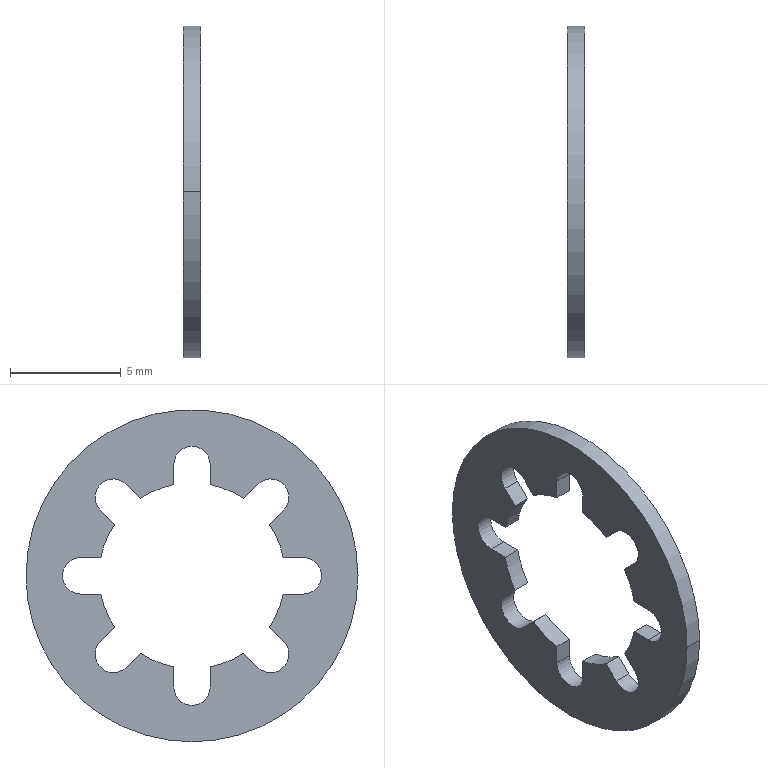Part | 1 solid | 36 faces | box 0.8 x 15 x 15 mm | volume 81.196 mm3 | cylinder 18 | plane 18 | commonest cylinder face diameters 1.65 x8 8.4 x8 15 x2
STEP:
#1=CARTESIAN_POINT('',(0.,0.,0.));
#2=DIRECTION('',(0.,0.,1.));
#3=DIRECTION('',(1.,0.,0.));
#4=AXIS2_PLACEMENT_3D('',#1,#2,#3);
#5=CARTESIAN_POINT('',(-282.773,180.5,-203.374));
#6=VERTEX_POINT('',#5);
#7=CARTESIAN_POINT('',(-283.573,180.5,-203.374));
#8=VERTEX_POINT('',#7);
#9=CARTESIAN_POINT('',(-282.773,180.5,-203.374));
#10=DIRECTION('',(-1.,0.,0.));
#11=VECTOR('',#10,1.);
#12=LINE('',#9,#11);
#13=EDGE_CURVE('',#6,#8,#12,.T.);
#14=ORIENTED_EDGE('',*,*,#13,.F.);
#15=CARTESIAN_POINT('',(-282.773,173.,-210.874));
#16=VERTEX_POINT('',#15);
#17=CARTESIAN_POINT('',(-282.773,173.,-203.374));
#18=DIRECTION('',(-1.,0.,0.));
#19=DIRECTION('',(0.,0.,-1.));
#20=AXIS2_PLACEMENT_3D('',#17,#18,#19);
#21=CIRCLE('',#20,7.5);
#22=EDGE_CURVE('',#6,#16,#21,.T.);
#23=ORIENTED_EDGE('',*,*,#22,.T.);
#24=CARTESIAN_POINT('',(-282.773,165.5,-203.374));
#25=VERTEX_POINT('',#24);
#26=CARTESIAN_POINT('',(-282.773,173.,-203.374));
#27=DIRECTION('',(-1.,0.,0.));
#28=DIRECTION('',(0.,0.,-1.));
#29=AXIS2_PLACEMENT_3D('',#26,#27,#28);
#30=CIRCLE('',#29,7.5);
#31=EDGE_CURVE('',#16,#25,#30,.T.);
#32=ORIENTED_EDGE('',*,*,#31,.T.);
#33=CARTESIAN_POINT('',(-283.573,165.5,-203.374));
#34=VERTEX_POINT('',#33);
#35=CARTESIAN_POINT('',(-282.773,165.5,-203.374));
#36=DIRECTION('',(-1.,0.,0.));
#37=VECTOR('',#36,1.);
#38=LINE('',#35,#37);
#39=EDGE_CURVE('',#25,#34,#38,.T.);
#40=ORIENTED_EDGE('',*,*,#39,.T.);
#41=CARTESIAN_POINT('',(-283.573,173.,-210.874));
#42=VERTEX_POINT('',#41);
#43=CARTESIAN_POINT('',(-283.573,173.,-203.374));
#44=DIRECTION('',(-1.,0.,0.));
#45=DIRECTION('',(0.,0.,-1.));
#46=AXIS2_PLACEMENT_3D('',#43,#44,#45);
#47=CIRCLE('',#46,7.5);
#48=EDGE_CURVE('',#42,#34,#47,.T.);
#49=ORIENTED_EDGE('',*,*,#48,.F.);
#50=CARTESIAN_POINT('',(-283.573,173.,-203.374));
#51=DIRECTION('',(-1.,0.,0.));
#52=DIRECTION('',(0.,0.,-1.));
#53=AXIS2_PLACEMENT_3D('',#50,#51,#52);
#54=CIRCLE('',#53,7.5);
#55=EDGE_CURVE('',#8,#42,#54,.T.);
#56=ORIENTED_EDGE('',*,*,#55,.F.);
#57=EDGE_LOOP('',(#14,#23,#32,#40,#49,#56));
#58=FACE_OUTER_BOUND('',#57,.T.);
#59=CARTESIAN_POINT('',(-283.573,173.,-203.374));
#60=DIRECTION('',(-1.,0.,0.));
#61=DIRECTION('',(0.,0.,1.));
#62=AXIS2_PLACEMENT_3D('',#59,#60,#61);
#63=CYLINDRICAL_SURFACE('',#62,7.5);
#64=ADVANCED_FACE('',(#58),#63,.T.);
#65=ORIENTED_EDGE('',*,*,#22,.F.);
#66=CARTESIAN_POINT('',(-282.773,173.,-203.374));
#67=DIRECTION('',(-1.,0.,0.));
#68=DIRECTION('',(0.,0.,-1.));
#69=AXIS2_PLACEMENT_3D('',#66,#67,#68);
#70=CIRCLE('',#69,7.5);
#71=EDGE_CURVE('',#25,#6,#70,.T.);
#72=ORIENTED_EDGE('',*,*,#71,.F.);
#73=ORIENTED_EDGE('',*,*,#31,.F.);
#74=EDGE_LOOP('',(#65,#72,#73));
#75=FACE_OUTER_BOUND('',#74,.T.);
#76=CARTESIAN_POINT('',(-282.773,172.175,-199.256));
#77=VERTEX_POINT('',#76);
#78=CARTESIAN_POINT('',(-282.773,170.671,-199.879));
#79=VERTEX_POINT('',#78);
#80=CARTESIAN_POINT('',(-282.773,173.,-203.374));
#81=DIRECTION('',(1.,0.,0.));
#82=DIRECTION('',(0.,-0.5544,0.8322));
#83=AXIS2_PLACEMENT_3D('',#80,#81,#82);
#84=CIRCLE('',#83,4.2);
#85=EDGE_CURVE('',#77,#79,#84,.T.);
#86=ORIENTED_EDGE('',*,*,#85,.F.);
#87=CARTESIAN_POINT('',(-282.773,172.175,-198.349));
#88=VERTEX_POINT('',#87);
#89=CARTESIAN_POINT('',(-282.773,172.175,-199.256));
#90=DIRECTION('',(0.,0.,-1.));
#91=VECTOR('',#90,1.);
#92=LINE('',#89,#91);
#93=EDGE_CURVE('',#88,#77,#92,.T.);
#94=ORIENTED_EDGE('',*,*,#93,.F.);
#95=CARTESIAN_POINT('',(-282.773,173.825,-198.349));
#96=VERTEX_POINT('',#95);
#97=CARTESIAN_POINT('',(-282.773,173.,-198.349));
#98=DIRECTION('',(1.,0.,0.));
#99=DIRECTION('',(0.,-1.,0.));
#100=AXIS2_PLACEMENT_3D('',#97,#98,#99);
#101=CIRCLE('',#100,0.825);
#102=EDGE_CURVE('',#96,#88,#101,.T.);
#103=ORIENTED_EDGE('',*,*,#102,.F.);
#104=CARTESIAN_POINT('',(-282.773,173.825,-199.256));
#105=VERTEX_POINT('',#104);
#106=CARTESIAN_POINT('',(-282.773,173.825,-198.349));
#107=DIRECTION('',(0.,0.,1.));
#108=VECTOR('',#107,1.);
#109=LINE('',#106,#108);
#110=EDGE_CURVE('',#105,#96,#109,.T.);
#111=ORIENTED_EDGE('',*,*,#110,.F.);
#112=CARTESIAN_POINT('',(-282.773,175.329,-199.879));
#113=VERTEX_POINT('',#112);
#114=CARTESIAN_POINT('',(-282.773,173.,-203.374));
#115=DIRECTION('',(1.,0.,0.));
#116=DIRECTION('',(0.,0.1964,0.9805));
#117=AXIS2_PLACEMENT_3D('',#114,#115,#116);
#118=CIRCLE('',#117,4.2);
#119=EDGE_CURVE('',#113,#105,#118,.T.);
#120=ORIENTED_EDGE('',*,*,#119,.F.);
#121=CARTESIAN_POINT('',(-282.773,175.97,-199.238));
#122=VERTEX_POINT('',#121);
#123=CARTESIAN_POINT('',(-282.773,175.329,-199.879));
#124=DIRECTION('',(0.,-0.7071,-0.7071));
#125=VECTOR('',#124,1.);
#126=LINE('',#123,#125);
#127=EDGE_CURVE('',#122,#113,#126,.T.);
#128=ORIENTED_EDGE('',*,*,#127,.F.);
#129=CARTESIAN_POINT('',(-282.773,177.137,-200.404));
#130=VERTEX_POINT('',#129);
#131=CARTESIAN_POINT('',(-282.773,176.553,-199.821));
#132=DIRECTION('',(1.,0.,0.));
#133=DIRECTION('',(0.,-0.7071,0.7071));
#134=AXIS2_PLACEMENT_3D('',#131,#132,#133);
#135=CIRCLE('',#134,0.825);
#136=EDGE_CURVE('',#130,#122,#135,.T.);
#137=ORIENTED_EDGE('',*,*,#136,.F.);
#138=CARTESIAN_POINT('',(-282.773,176.495,-201.046));
#139=VERTEX_POINT('',#138);
#140=CARTESIAN_POINT('',(-282.773,177.137,-200.404));
#141=DIRECTION('',(0.,0.7071,0.7071));
#142=VECTOR('',#141,1.);
#143=LINE('',#140,#142);
#144=EDGE_CURVE('',#139,#130,#143,.T.);
#145=ORIENTED_EDGE('',*,*,#144,.F.);
#146=CARTESIAN_POINT('',(-282.773,177.118,-202.549));
#147=VERTEX_POINT('',#146);
#148=CARTESIAN_POINT('',(-282.773,173.,-203.374));
#149=DIRECTION('',(1.,0.,0.));
#150=DIRECTION('',(0.,0.8322,0.5544));
#151=AXIS2_PLACEMENT_3D('',#148,#149,#150);
#152=CIRCLE('',#151,4.2);
#153=EDGE_CURVE('',#147,#139,#152,.T.);
#154=ORIENTED_EDGE('',*,*,#153,.F.);
#155=CARTESIAN_POINT('',(-282.773,178.025,-202.549));
#156=VERTEX_POINT('',#155);
#157=CARTESIAN_POINT('',(-282.773,177.118,-202.549));
#158=DIRECTION('',(0.,-1.,0.));
#159=VECTOR('',#158,1.);
#160=LINE('',#157,#159);
#161=EDGE_CURVE('',#156,#147,#160,.T.);
#162=ORIENTED_EDGE('',*,*,#161,.F.);
#163=CARTESIAN_POINT('',(-282.773,178.025,-204.199));
#164=VERTEX_POINT('',#163);
#165=CARTESIAN_POINT('',(-282.773,178.025,-203.374));
#166=DIRECTION('',(1.,0.,0.));
#167=DIRECTION('',(0.,0.,1.));
#168=AXIS2_PLACEMENT_3D('',#165,#166,#167);
#169=CIRCLE('',#168,0.825);
#170=EDGE_CURVE('',#164,#156,#169,.T.);
#171=ORIENTED_EDGE('',*,*,#170,.F.);
#172=CARTESIAN_POINT('',(-282.773,177.118,-204.199));
#173=VERTEX_POINT('',#172);
#174=CARTESIAN_POINT('',(-282.773,178.025,-204.199));
#175=DIRECTION('',(0.,1.,0.));
#176=VECTOR('',#175,1.);
#177=LINE('',#174,#176);
#178=EDGE_CURVE('',#173,#164,#177,.T.);
#179=ORIENTED_EDGE('',*,*,#178,.F.);
#180=CARTESIAN_POINT('',(-282.773,176.495,-205.703));
#181=VERTEX_POINT('',#180);
#182=CARTESIAN_POINT('',(-282.773,173.,-203.374));
#183=DIRECTION('',(1.,0.,0.));
#184=DIRECTION('',(0.,0.9805,-0.1964));
#185=AXIS2_PLACEMENT_3D('',#182,#183,#184);
#186=CIRCLE('',#185,4.2);
#187=EDGE_CURVE('',#181,#173,#186,.T.);
#188=ORIENTED_EDGE('',*,*,#187,.F.);
#189=CARTESIAN_POINT('',(-282.773,177.137,-206.344));
#190=VERTEX_POINT('',#189);
#191=CARTESIAN_POINT('',(-282.773,176.495,-205.703));
#192=DIRECTION('',(0.,-0.7071,0.7071));
#193=VECTOR('',#192,1.);
#194=LINE('',#191,#193);
#195=EDGE_CURVE('',#190,#181,#194,.T.);
#196=ORIENTED_EDGE('',*,*,#195,.F.);
#197=CARTESIAN_POINT('',(-282.773,175.97,-207.511));
#198=VERTEX_POINT('',#197);
#199=CARTESIAN_POINT('',(-282.773,176.553,-206.927));
#200=DIRECTION('',(1.,0.,0.));
#201=DIRECTION('',(0.,0.7071,0.7071));
#202=AXIS2_PLACEMENT_3D('',#199,#200,#201);
#203=CIRCLE('',#202,0.825);
#204=EDGE_CURVE('',#198,#190,#203,.T.);
#205=ORIENTED_EDGE('',*,*,#204,.F.);
#206=CARTESIAN_POINT('',(-282.773,175.329,-206.87));
#207=VERTEX_POINT('',#206);
#208=CARTESIAN_POINT('',(-282.773,175.97,-207.511));
#209=DIRECTION('',(0.,0.7071,-0.7071));
#210=VECTOR('',#209,1.);
#211=LINE('',#208,#210);
#212=EDGE_CURVE('',#207,#198,#211,.T.);
#213=ORIENTED_EDGE('',*,*,#212,.F.);
#214=CARTESIAN_POINT('',(-282.773,173.825,-207.492));
#215=VERTEX_POINT('',#214);
#216=CARTESIAN_POINT('',(-282.773,173.,-203.374));
#217=DIRECTION('',(1.,0.,0.));
#218=DIRECTION('',(0.,0.5544,-0.8322));
#219=AXIS2_PLACEMENT_3D('',#216,#217,#218);
#220=CIRCLE('',#219,4.2);
#221=EDGE_CURVE('',#215,#207,#220,.T.);
#222=ORIENTED_EDGE('',*,*,#221,.F.);
#223=CARTESIAN_POINT('',(-282.773,173.825,-208.399));
#224=VERTEX_POINT('',#223);
#225=CARTESIAN_POINT('',(-282.773,173.825,-207.492));
#226=DIRECTION('',(0.,0.,1.));
#227=VECTOR('',#226,1.);
#228=LINE('',#225,#227);
#229=EDGE_CURVE('',#224,#215,#228,.T.);
#230=ORIENTED_EDGE('',*,*,#229,.F.);
#231=CARTESIAN_POINT('',(-282.773,172.175,-208.399));
#232=VERTEX_POINT('',#231);
#233=CARTESIAN_POINT('',(-282.773,173.,-208.399));
#234=DIRECTION('',(1.,0.,0.));
#235=DIRECTION('',(0.,1.,0.));
#236=AXIS2_PLACEMENT_3D('',#233,#234,#235);
#237=CIRCLE('',#236,0.825);
#238=EDGE_CURVE('',#232,#224,#237,.T.);
#239=ORIENTED_EDGE('',*,*,#238,.F.);
#240=CARTESIAN_POINT('',(-282.773,172.175,-207.492));
#241=VERTEX_POINT('',#240);
#242=CARTESIAN_POINT('',(-282.773,172.175,-208.399));
#243=DIRECTION('',(0.,0.,-1.));
#244=VECTOR('',#243,1.);
#245=LINE('',#242,#244);
#246=EDGE_CURVE('',#241,#232,#245,.T.);
#247=ORIENTED_EDGE('',*,*,#246,.F.);
#248=CARTESIAN_POINT('',(-282.773,170.671,-206.87));
#249=VERTEX_POINT('',#248);
#250=CARTESIAN_POINT('',(-282.773,173.,-203.374));
#251=DIRECTION('',(1.,0.,0.));
#252=DIRECTION('',(0.,-0.1964,-0.9805));
#253=AXIS2_PLACEMENT_3D('',#250,#251,#252);
#254=CIRCLE('',#253,4.2);
#255=EDGE_CURVE('',#249,#241,#254,.T.);
#256=ORIENTED_EDGE('',*,*,#255,.F.);
#257=CARTESIAN_POINT('',(-282.773,170.03,-207.511));
#258=VERTEX_POINT('',#257);
#259=CARTESIAN_POINT('',(-282.773,170.671,-206.87));
#260=DIRECTION('',(0.,0.7071,0.7071));
#261=VECTOR('',#260,1.);
#262=LINE('',#259,#261);
#263=EDGE_CURVE('',#258,#249,#262,.T.);
#264=ORIENTED_EDGE('',*,*,#263,.F.);
#265=CARTESIAN_POINT('',(-282.773,168.863,-206.344));
#266=VERTEX_POINT('',#265);
#267=CARTESIAN_POINT('',(-282.773,169.447,-206.927));
#268=DIRECTION('',(1.,0.,0.));
#269=DIRECTION('',(0.,0.7071,-0.7071));
#270=AXIS2_PLACEMENT_3D('',#267,#268,#269);
#271=CIRCLE('',#270,0.825);
#272=EDGE_CURVE('',#266,#258,#271,.T.);
#273=ORIENTED_EDGE('',*,*,#272,.F.);
#274=CARTESIAN_POINT('',(-282.773,169.505,-205.703));
#275=VERTEX_POINT('',#274);
#276=CARTESIAN_POINT('',(-282.773,168.863,-206.344));
#277=DIRECTION('',(0.,-0.7071,-0.7071));
#278=VECTOR('',#277,1.);
#279=LINE('',#276,#278);
#280=EDGE_CURVE('',#275,#266,#279,.T.);
#281=ORIENTED_EDGE('',*,*,#280,.F.);
#282=CARTESIAN_POINT('',(-282.773,168.882,-204.199));
#283=VERTEX_POINT('',#282);
#284=CARTESIAN_POINT('',(-282.773,173.,-203.374));
#285=DIRECTION('',(1.,0.,0.));
#286=DIRECTION('',(0.,-0.8322,-0.5544));
#287=AXIS2_PLACEMENT_3D('',#284,#285,#286);
#288=CIRCLE('',#287,4.2);
#289=EDGE_CURVE('',#283,#275,#288,.T.);
#290=ORIENTED_EDGE('',*,*,#289,.F.);
#291=CARTESIAN_POINT('',(-282.773,167.975,-204.199));
#292=VERTEX_POINT('',#291);
#293=CARTESIAN_POINT('',(-282.773,168.882,-204.199));
#294=DIRECTION('',(0.,1.,0.));
#295=VECTOR('',#294,1.);
#296=LINE('',#293,#295);
#297=EDGE_CURVE('',#292,#283,#296,.T.);
#298=ORIENTED_EDGE('',*,*,#297,.F.);
#299=CARTESIAN_POINT('',(-282.773,167.975,-202.549));
#300=VERTEX_POINT('',#299);
#301=CARTESIAN_POINT('',(-282.773,167.975,-203.374));
#302=DIRECTION('',(1.,0.,0.));
#303=DIRECTION('',(0.,0.,-1.));
#304=AXIS2_PLACEMENT_3D('',#301,#302,#303);
#305=CIRCLE('',#304,0.825);
#306=EDGE_CURVE('',#300,#292,#305,.T.);
#307=ORIENTED_EDGE('',*,*,#306,.F.);
#308=CARTESIAN_POINT('',(-282.773,168.882,-202.549));
#309=VERTEX_POINT('',#308);
#310=CARTESIAN_POINT('',(-282.773,167.975,-202.549));
#311=DIRECTION('',(0.,-1.,0.));
#312=VECTOR('',#311,1.);
#313=LINE('',#310,#312);
#314=EDGE_CURVE('',#309,#300,#313,.T.);
#315=ORIENTED_EDGE('',*,*,#314,.F.);
#316=CARTESIAN_POINT('',(-282.773,169.505,-201.046));
#317=VERTEX_POINT('',#316);
#318=CARTESIAN_POINT('',(-282.773,173.,-203.374));
#319=DIRECTION('',(1.,0.,0.));
#320=DIRECTION('',(0.,-0.9805,0.1964));
#321=AXIS2_PLACEMENT_3D('',#318,#319,#320);
#322=CIRCLE('',#321,4.2);
#323=EDGE_CURVE('',#317,#309,#322,.T.);
#324=ORIENTED_EDGE('',*,*,#323,.F.);
#325=CARTESIAN_POINT('',(-282.773,168.863,-200.404));
#326=VERTEX_POINT('',#325);
#327=CARTESIAN_POINT('',(-282.773,169.505,-201.046));
#328=DIRECTION('',(0.,0.7071,-0.7071));
#329=VECTOR('',#328,1.);
#330=LINE('',#327,#329);
#331=EDGE_CURVE('',#326,#317,#330,.T.);
#332=ORIENTED_EDGE('',*,*,#331,.F.);
#333=CARTESIAN_POINT('',(-282.773,170.03,-199.238));
#334=VERTEX_POINT('',#333);
#335=CARTESIAN_POINT('',(-282.773,169.447,-199.821));
#336=DIRECTION('',(1.,0.,0.));
#337=DIRECTION('',(0.,-0.7071,-0.7071));
#338=AXIS2_PLACEMENT_3D('',#335,#336,#337);
#339=CIRCLE('',#338,0.825);
#340=EDGE_CURVE('',#334,#326,#339,.T.);
#341=ORIENTED_EDGE('',*,*,#340,.F.);
#342=CARTESIAN_POINT('',(-282.773,170.03,-199.238));
#343=DIRECTION('',(0.,-0.7071,0.7071));
#344=VECTOR('',#343,1.);
#345=LINE('',#342,#344);
#346=EDGE_CURVE('',#79,#334,#345,.T.);
#347=ORIENTED_EDGE('',*,*,#346,.F.);
#348=EDGE_LOOP('',(#86,#94,#103,#111,#120,#128,#137,#145,#154,#162,#171,#179,#188,#196,#205,#213,#222,#230,#239,#247,#256,#264,#273,#281,#290,#298,#307,#315,#324,#332,#341,#347));
#349=FACE_BOUND('',#348,.T.);
#350=CARTESIAN_POINT('',(-282.773,173.,-203.374));
#351=DIRECTION('',(-1.,0.,0.));
#352=DIRECTION('',(0.,0.,-1.));
#353=AXIS2_PLACEMENT_3D('',#350,#351,#352);
#354=PLANE('',#353);
#355=ADVANCED_FACE('',(#75,#349),#354,.F.);
#356=ORIENTED_EDGE('',*,*,#346,.T.);
#357=CARTESIAN_POINT('',(-283.573,170.03,-199.238));
#358=VERTEX_POINT('',#357);
#359=CARTESIAN_POINT('',(-283.573,170.03,-199.238));
#360=DIRECTION('',(1.,0.,0.));
#361=VECTOR('',#360,1.);
#362=LINE('',#359,#361);
#363=EDGE_CURVE('',#358,#334,#362,.T.);
#364=ORIENTED_EDGE('',*,*,#363,.F.);
#365=CARTESIAN_POINT('',(-283.573,170.671,-199.879));
#366=VERTEX_POINT('',#365);
#367=CARTESIAN_POINT('',(-283.573,170.03,-199.238));
#368=DIRECTION('',(0.,0.7071,-0.7071));
#369=VECTOR('',#368,1.);
#370=LINE('',#367,#369);
#371=EDGE_CURVE('',#358,#366,#370,.T.);
#372=ORIENTED_EDGE('',*,*,#371,.T.);
#373=CARTESIAN_POINT('',(-283.573,170.671,-199.879));
#374=DIRECTION('',(1.,0.,0.));
#375=VECTOR('',#374,1.);
#376=LINE('',#373,#375);
#377=EDGE_CURVE('',#366,#79,#376,.T.);
#378=ORIENTED_EDGE('',*,*,#377,.T.);
#379=EDGE_LOOP('',(#356,#364,#372,#378));
#380=FACE_OUTER_BOUND('',#379,.T.);
#381=CARTESIAN_POINT('',(-283.573,170.671,-199.879));
#382=DIRECTION('',(0.,-0.7071,-0.7071));
#383=DIRECTION('',(0.,0.7071,-0.7071));
#384=AXIS2_PLACEMENT_3D('',#381,#382,#383);
#385=PLANE('',#384);
#386=ADVANCED_FACE('',(#380),#385,.T.);
#387=ORIENTED_EDGE('',*,*,#85,.T.);
#388=ORIENTED_EDGE('',*,*,#377,.F.);
#389=CARTESIAN_POINT('',(-283.573,172.175,-199.256));
#390=VERTEX_POINT('',#389);
#391=CARTESIAN_POINT('',(-283.573,173.,-203.374));
#392=DIRECTION('',(-1.,0.,0.));
#393=DIRECTION('',(0.,-0.5544,0.8322));
#394=AXIS2_PLACEMENT_3D('',#391,#392,#393);
#395=CIRCLE('',#394,4.2);
#396=EDGE_CURVE('',#366,#390,#395,.T.);
#397=ORIENTED_EDGE('',*,*,#396,.T.);
#398=CARTESIAN_POINT('',(-283.573,172.175,-199.256));
#399=DIRECTION('',(1.,0.,0.));
#400=VECTOR('',#399,1.);
#401=LINE('',#398,#400);
#402=EDGE_CURVE('',#390,#77,#401,.T.);
#403=ORIENTED_EDGE('',*,*,#402,.T.);
#404=EDGE_LOOP('',(#387,#388,#397,#403));
#405=FACE_OUTER_BOUND('',#404,.T.);
#406=CARTESIAN_POINT('',(-283.573,173.,-203.374));
#407=DIRECTION('',(-1.,0.,0.));
#408=DIRECTION('',(0.,0.3827,-0.9239));
#409=AXIS2_PLACEMENT_3D('',#406,#407,#408);
#410=CYLINDRICAL_SURFACE('',#409,4.2);
#411=ADVANCED_FACE('',(#405),#410,.F.);
#412=ORIENTED_EDGE('',*,*,#93,.T.);
#413=ORIENTED_EDGE('',*,*,#402,.F.);
#414=CARTESIAN_POINT('',(-283.573,172.175,-198.349));
#415=VERTEX_POINT('',#414);
#416=CARTESIAN_POINT('',(-283.573,172.175,-199.256));
#417=DIRECTION('',(0.,0.,1.));
#418=VECTOR('',#417,1.);
#419=LINE('',#416,#418);
#420=EDGE_CURVE('',#390,#415,#419,.T.);
#421=ORIENTED_EDGE('',*,*,#420,.T.);
#422=CARTESIAN_POINT('',(-283.573,172.175,-198.349));
#423=DIRECTION('',(1.,0.,0.));
#424=VECTOR('',#423,1.);
#425=LINE('',#422,#424);
#426=EDGE_CURVE('',#415,#88,#425,.T.);
#427=ORIENTED_EDGE('',*,*,#426,.T.);
#428=EDGE_LOOP('',(#412,#413,#421,#427));
#429=FACE_OUTER_BOUND('',#428,.T.);
#430=CARTESIAN_POINT('',(-283.573,172.175,-198.349));
#431=DIRECTION('',(0.,1.,0.));
#432=DIRECTION('',(0.,0.,1.));
#433=AXIS2_PLACEMENT_3D('',#430,#431,#432);
#434=PLANE('',#433);
#435=ADVANCED_FACE('',(#429),#434,.T.);
#436=ORIENTED_EDGE('',*,*,#102,.T.);
#437=ORIENTED_EDGE('',*,*,#426,.F.);
#438=CARTESIAN_POINT('',(-283.573,173.825,-198.349));
#439=VERTEX_POINT('',#438);
#440=CARTESIAN_POINT('',(-283.573,173.,-198.349));
#441=DIRECTION('',(-1.,0.,0.));
#442=DIRECTION('',(0.,-1.,0.));
#443=AXIS2_PLACEMENT_3D('',#440,#441,#442);
#444=CIRCLE('',#443,0.825);
#445=EDGE_CURVE('',#415,#439,#444,.T.);
#446=ORIENTED_EDGE('',*,*,#445,.T.);
#447=CARTESIAN_POINT('',(-283.573,173.825,-198.349));
#448=DIRECTION('',(1.,0.,0.));
#449=VECTOR('',#448,1.);
#450=LINE('',#447,#449);
#451=EDGE_CURVE('',#439,#96,#450,.T.);
#452=ORIENTED_EDGE('',*,*,#451,.T.);
#453=EDGE_LOOP('',(#436,#437,#446,#452));
#454=FACE_OUTER_BOUND('',#453,.T.);
#455=CARTESIAN_POINT('',(-283.573,173.,-198.349));
#456=DIRECTION('',(-1.,0.,0.));
#457=DIRECTION('',(0.,0.,-1.));
#458=AXIS2_PLACEMENT_3D('',#455,#456,#457);
#459=CYLINDRICAL_SURFACE('',#458,0.825);
#460=ADVANCED_FACE('',(#454),#459,.F.);
#461=ORIENTED_EDGE('',*,*,#110,.T.);
#462=ORIENTED_EDGE('',*,*,#451,.F.);
#463=CARTESIAN_POINT('',(-283.573,173.825,-199.256));
#464=VERTEX_POINT('',#463);
#465=CARTESIAN_POINT('',(-283.573,173.825,-198.349));
#466=DIRECTION('',(0.,0.,-1.));
#467=VECTOR('',#466,1.);
#468=LINE('',#465,#467);
#469=EDGE_CURVE('',#439,#464,#468,.T.);
#470=ORIENTED_EDGE('',*,*,#469,.T.);
#471=CARTESIAN_POINT('',(-283.573,173.825,-199.256));
#472=DIRECTION('',(1.,0.,0.));
#473=VECTOR('',#472,1.);
#474=LINE('',#471,#473);
#475=EDGE_CURVE('',#464,#105,#474,.T.);
#476=ORIENTED_EDGE('',*,*,#475,.T.);
#477=EDGE_LOOP('',(#461,#462,#470,#476));
#478=FACE_OUTER_BOUND('',#477,.T.);
#479=CARTESIAN_POINT('',(-283.573,173.825,-199.256));
#480=DIRECTION('',(0.,-1.,0.));
#481=DIRECTION('',(0.,0.,-1.));
#482=AXIS2_PLACEMENT_3D('',#479,#480,#481);
#483=PLANE('',#482);
#484=ADVANCED_FACE('',(#478),#483,.T.);
#485=ORIENTED_EDGE('',*,*,#119,.T.);
#486=ORIENTED_EDGE('',*,*,#475,.F.);
#487=CARTESIAN_POINT('',(-283.573,175.329,-199.879));
#488=VERTEX_POINT('',#487);
#489=CARTESIAN_POINT('',(-283.573,173.,-203.374));
#490=DIRECTION('',(-1.,0.,0.));
#491=DIRECTION('',(0.,0.1964,0.9805));
#492=AXIS2_PLACEMENT_3D('',#489,#490,#491);
#493=CIRCLE('',#492,4.2);
#494=EDGE_CURVE('',#464,#488,#493,.T.);
#495=ORIENTED_EDGE('',*,*,#494,.T.);
#496=CARTESIAN_POINT('',(-283.573,175.329,-199.879));
#497=DIRECTION('',(1.,0.,0.));
#498=VECTOR('',#497,1.);
#499=LINE('',#496,#498);
#500=EDGE_CURVE('',#488,#113,#499,.T.);
#501=ORIENTED_EDGE('',*,*,#500,.T.);
#502=EDGE_LOOP('',(#485,#486,#495,#501));
#503=FACE_OUTER_BOUND('',#502,.T.);
#504=CARTESIAN_POINT('',(-283.573,173.,-203.374));
#505=DIRECTION('',(-1.,0.,0.));
#506=DIRECTION('',(0.,-0.3827,-0.9239));
#507=AXIS2_PLACEMENT_3D('',#504,#505,#506);
#508=CYLINDRICAL_SURFACE('',#507,4.2);
#509=ADVANCED_FACE('',(#503),#508,.F.);
#510=ORIENTED_EDGE('',*,*,#127,.T.);
#511=ORIENTED_EDGE('',*,*,#500,.F.);
#512=CARTESIAN_POINT('',(-283.573,175.97,-199.238));
#513=VERTEX_POINT('',#512);
#514=CARTESIAN_POINT('',(-283.573,175.329,-199.879));
#515=DIRECTION('',(0.,0.7071,0.7071));
#516=VECTOR('',#515,1.);
#517=LINE('',#514,#516);
#518=EDGE_CURVE('',#488,#513,#517,.T.);
#519=ORIENTED_EDGE('',*,*,#518,.T.);
#520=CARTESIAN_POINT('',(-283.573,175.97,-199.238));
#521=DIRECTION('',(1.,0.,0.));
#522=VECTOR('',#521,1.);
#523=LINE('',#520,#522);
#524=EDGE_CURVE('',#513,#122,#523,.T.);
#525=ORIENTED_EDGE('',*,*,#524,.T.);
#526=EDGE_LOOP('',(#510,#511,#519,#525));
#527=FACE_OUTER_BOUND('',#526,.T.);
#528=CARTESIAN_POINT('',(-283.573,175.97,-199.238));
#529=DIRECTION('',(0.,0.7071,-0.7071));
#530=DIRECTION('',(0.,0.7071,0.7071));
#531=AXIS2_PLACEMENT_3D('',#528,#529,#530);
#532=PLANE('',#531);
#533=ADVANCED_FACE('',(#527),#532,.T.);
#534=ORIENTED_EDGE('',*,*,#136,.T.);
#535=ORIENTED_EDGE('',*,*,#524,.F.);
#536=CARTESIAN_POINT('',(-283.573,177.137,-200.404));
#537=VERTEX_POINT('',#536);
#538=CARTESIAN_POINT('',(-283.573,176.553,-199.821));
#539=DIRECTION('',(-1.,0.,0.));
#540=DIRECTION('',(0.,-0.7071,0.7071));
#541=AXIS2_PLACEMENT_3D('',#538,#539,#540);
#542=CIRCLE('',#541,0.825);
#543=EDGE_CURVE('',#513,#537,#542,.T.);
#544=ORIENTED_EDGE('',*,*,#543,.T.);
#545=CARTESIAN_POINT('',(-283.573,177.137,-200.404));
#546=DIRECTION('',(1.,0.,0.));
#547=VECTOR('',#546,1.);
#548=LINE('',#545,#547);
#549=EDGE_CURVE('',#537,#130,#548,.T.);
#550=ORIENTED_EDGE('',*,*,#549,.T.);
#551=EDGE_LOOP('',(#534,#535,#544,#550));
#552=FACE_OUTER_BOUND('',#551,.T.);
#553=CARTESIAN_POINT('',(-283.573,176.553,-199.821));
#554=DIRECTION('',(-1.,0.,0.));
#555=DIRECTION('',(0.,-0.7071,-0.7071));
#556=AXIS2_PLACEMENT_3D('',#553,#554,#555);
#557=CYLINDRICAL_SURFACE('',#556,0.825);
#558=ADVANCED_FACE('',(#552),#557,.F.);
#559=ORIENTED_EDGE('',*,*,#144,.T.);
#560=ORIENTED_EDGE('',*,*,#549,.F.);
#561=CARTESIAN_POINT('',(-283.573,176.495,-201.046));
#562=VERTEX_POINT('',#561);
#563=CARTESIAN_POINT('',(-283.573,177.137,-200.404));
#564=DIRECTION('',(0.,-0.7071,-0.7071));
#565=VECTOR('',#564,1.);
#566=LINE('',#563,#565);
#567=EDGE_CURVE('',#537,#562,#566,.T.);
#568=ORIENTED_EDGE('',*,*,#567,.T.);
#569=CARTESIAN_POINT('',(-283.573,176.495,-201.046));
#570=DIRECTION('',(1.,0.,0.));
#571=VECTOR('',#570,1.);
#572=LINE('',#569,#571);
#573=EDGE_CURVE('',#562,#139,#572,.T.);
#574=ORIENTED_EDGE('',*,*,#573,.T.);
#575=EDGE_LOOP('',(#559,#560,#568,#574));
#576=FACE_OUTER_BOUND('',#575,.T.);
#577=CARTESIAN_POINT('',(-283.573,176.495,-201.046));
#578=DIRECTION('',(0.,-0.7071,0.7071));
#579=DIRECTION('',(0.,-0.7071,-0.7071));
#580=AXIS2_PLACEMENT_3D('',#577,#578,#579);
#581=PLANE('',#580);
#582=ADVANCED_FACE('',(#576),#581,.T.);
#583=ORIENTED_EDGE('',*,*,#153,.T.);
#584=ORIENTED_EDGE('',*,*,#573,.F.);
#585=CARTESIAN_POINT('',(-283.573,177.118,-202.549));
#586=VERTEX_POINT('',#585);
#587=CARTESIAN_POINT('',(-283.573,173.,-203.374));
#588=DIRECTION('',(-1.,0.,0.));
#589=DIRECTION('',(0.,0.8322,0.5544));
#590=AXIS2_PLACEMENT_3D('',#587,#588,#589);
#591=CIRCLE('',#590,4.2);
#592=EDGE_CURVE('',#562,#586,#591,.T.);
#593=ORIENTED_EDGE('',*,*,#592,.T.);
#594=CARTESIAN_POINT('',(-283.573,177.118,-202.549));
#595=DIRECTION('',(1.,0.,0.));
#596=VECTOR('',#595,1.);
#597=LINE('',#594,#596);
#598=EDGE_CURVE('',#586,#147,#597,.T.);
#599=ORIENTED_EDGE('',*,*,#598,.T.);
#600=EDGE_LOOP('',(#583,#584,#593,#599));
#601=FACE_OUTER_BOUND('',#600,.T.);
#602=CARTESIAN_POINT('',(-283.573,173.,-203.374));
#603=DIRECTION('',(-1.,0.,0.));
#604=DIRECTION('',(0.,-0.9239,-0.3827));
#605=AXIS2_PLACEMENT_3D('',#602,#603,#604);
#606=CYLINDRICAL_SURFACE('',#605,4.2);
#607=ADVANCED_FACE('',(#601),#606,.F.);
#608=ORIENTED_EDGE('',*,*,#161,.T.);
#609=ORIENTED_EDGE('',*,*,#598,.F.);
#610=CARTESIAN_POINT('',(-283.573,178.025,-202.549));
#611=VERTEX_POINT('',#610);
#612=CARTESIAN_POINT('',(-283.573,177.118,-202.549));
#613=DIRECTION('',(0.,1.,0.));
#614=VECTOR('',#613,1.);
#615=LINE('',#612,#614);
#616=EDGE_CURVE('',#586,#611,#615,.T.);
#617=ORIENTED_EDGE('',*,*,#616,.T.);
#618=CARTESIAN_POINT('',(-283.573,178.025,-202.549));
#619=DIRECTION('',(1.,0.,0.));
#620=VECTOR('',#619,1.);
#621=LINE('',#618,#620);
#622=EDGE_CURVE('',#611,#156,#621,.T.);
#623=ORIENTED_EDGE('',*,*,#622,.T.);
#624=EDGE_LOOP('',(#608,#609,#617,#623));
#625=FACE_OUTER_BOUND('',#624,.T.);
#626=CARTESIAN_POINT('',(-283.573,178.025,-202.549));
#627=DIRECTION('',(0.,0.,-1.));
#628=DIRECTION('',(0.,1.,0.));
#629=AXIS2_PLACEMENT_3D('',#626,#627,#628);
#630=PLANE('',#629);
#631=ADVANCED_FACE('',(#625),#630,.T.);
#632=ORIENTED_EDGE('',*,*,#170,.T.);
#633=ORIENTED_EDGE('',*,*,#622,.F.);
#634=CARTESIAN_POINT('',(-283.573,178.025,-204.199));
#635=VERTEX_POINT('',#634);
#636=CARTESIAN_POINT('',(-283.573,178.025,-203.374));
#637=DIRECTION('',(-1.,0.,0.));
#638=DIRECTION('',(0.,0.,1.));
#639=AXIS2_PLACEMENT_3D('',#636,#637,#638);
#640=CIRCLE('',#639,0.825);
#641=EDGE_CURVE('',#611,#635,#640,.T.);
#642=ORIENTED_EDGE('',*,*,#641,.T.);
#643=CARTESIAN_POINT('',(-283.573,178.025,-204.199));
#644=DIRECTION('',(1.,0.,0.));
#645=VECTOR('',#644,1.);
#646=LINE('',#643,#645);
#647=EDGE_CURVE('',#635,#164,#646,.T.);
#648=ORIENTED_EDGE('',*,*,#647,.T.);
#649=EDGE_LOOP('',(#632,#633,#642,#648));
#650=FACE_OUTER_BOUND('',#649,.T.);
#651=CARTESIAN_POINT('',(-283.573,178.025,-203.374));
#652=DIRECTION('',(-1.,0.,0.));
#653=DIRECTION('',(0.,-1.,0.));
#654=AXIS2_PLACEMENT_3D('',#651,#652,#653);
#655=CYLINDRICAL_SURFACE('',#654,0.825);
#656=ADVANCED_FACE('',(#650),#655,.F.);
#657=ORIENTED_EDGE('',*,*,#178,.T.);
#658=ORIENTED_EDGE('',*,*,#647,.F.);
#659=CARTESIAN_POINT('',(-283.573,177.118,-204.199));
#660=VERTEX_POINT('',#659);
#661=CARTESIAN_POINT('',(-283.573,178.025,-204.199));
#662=DIRECTION('',(0.,-1.,0.));
#663=VECTOR('',#662,1.);
#664=LINE('',#661,#663);
#665=EDGE_CURVE('',#635,#660,#664,.T.);
#666=ORIENTED_EDGE('',*,*,#665,.T.);
#667=CARTESIAN_POINT('',(-283.573,177.118,-204.199));
#668=DIRECTION('',(1.,0.,0.));
#669=VECTOR('',#668,1.);
#670=LINE('',#667,#669);
#671=EDGE_CURVE('',#660,#173,#670,.T.);
#672=ORIENTED_EDGE('',*,*,#671,.T.);
#673=EDGE_LOOP('',(#657,#658,#666,#672));
#674=FACE_OUTER_BOUND('',#673,.T.);
#675=CARTESIAN_POINT('',(-283.573,177.118,-204.199));
#676=DIRECTION('',(0.,0.,1.));
#677=DIRECTION('',(0.,-1.,0.));
#678=AXIS2_PLACEMENT_3D('',#675,#676,#677);
#679=PLANE('',#678);
#680=ADVANCED_FACE('',(#674),#679,.T.);
#681=ORIENTED_EDGE('',*,*,#187,.T.);
#682=ORIENTED_EDGE('',*,*,#671,.F.);
#683=CARTESIAN_POINT('',(-283.573,176.495,-205.703));
#684=VERTEX_POINT('',#683);
#685=CARTESIAN_POINT('',(-283.573,173.,-203.374));
#686=DIRECTION('',(-1.,0.,0.));
#687=DIRECTION('',(0.,0.9805,-0.1964));
#688=AXIS2_PLACEMENT_3D('',#685,#686,#687);
#689=CIRCLE('',#688,4.2);
#690=EDGE_CURVE('',#660,#684,#689,.T.);
#691=ORIENTED_EDGE('',*,*,#690,.T.);
#692=CARTESIAN_POINT('',(-283.573,176.495,-205.703));
#693=DIRECTION('',(1.,0.,0.));
#694=VECTOR('',#693,1.);
#695=LINE('',#692,#694);
#696=EDGE_CURVE('',#684,#181,#695,.T.);
#697=ORIENTED_EDGE('',*,*,#696,.T.);
#698=EDGE_LOOP('',(#681,#682,#691,#697));
#699=FACE_OUTER_BOUND('',#698,.T.);
#700=CARTESIAN_POINT('',(-283.573,173.,-203.374));
#701=DIRECTION('',(-1.,0.,0.));
#702=DIRECTION('',(0.,-0.9239,0.3827));
#703=AXIS2_PLACEMENT_3D('',#700,#701,#702);
#704=CYLINDRICAL_SURFACE('',#703,4.2);
#705=ADVANCED_FACE('',(#699),#704,.F.);
#706=ORIENTED_EDGE('',*,*,#195,.T.);
#707=ORIENTED_EDGE('',*,*,#696,.F.);
#708=CARTESIAN_POINT('',(-283.573,177.137,-206.344));
#709=VERTEX_POINT('',#708);
#710=CARTESIAN_POINT('',(-283.573,176.495,-205.703));
#711=DIRECTION('',(0.,0.7071,-0.7071));
#712=VECTOR('',#711,1.);
#713=LINE('',#710,#712);
#714=EDGE_CURVE('',#684,#709,#713,.T.);
#715=ORIENTED_EDGE('',*,*,#714,.T.);
#716=CARTESIAN_POINT('',(-283.573,177.137,-206.344));
#717=DIRECTION('',(1.,0.,0.));
#718=VECTOR('',#717,1.);
#719=LINE('',#716,#718);
#720=EDGE_CURVE('',#709,#190,#719,.T.);
#721=ORIENTED_EDGE('',*,*,#720,.T.);
#722=EDGE_LOOP('',(#706,#707,#715,#721));
#723=FACE_OUTER_BOUND('',#722,.T.);
#724=CARTESIAN_POINT('',(-283.573,177.137,-206.344));
#725=DIRECTION('',(0.,-0.7071,-0.7071));
#726=DIRECTION('',(0.,0.7071,-0.7071));
#727=AXIS2_PLACEMENT_3D('',#724,#725,#726);
#728=PLANE('',#727);
#729=ADVANCED_FACE('',(#723),#728,.T.);
#730=ORIENTED_EDGE('',*,*,#204,.T.);
#731=ORIENTED_EDGE('',*,*,#720,.F.);
#732=CARTESIAN_POINT('',(-283.573,175.97,-207.511));
#733=VERTEX_POINT('',#732);
#734=CARTESIAN_POINT('',(-283.573,176.553,-206.927));
#735=DIRECTION('',(-1.,0.,0.));
#736=DIRECTION('',(0.,0.7071,0.7071));
#737=AXIS2_PLACEMENT_3D('',#734,#735,#736);
#738=CIRCLE('',#737,0.825);
#739=EDGE_CURVE('',#709,#733,#738,.T.);
#740=ORIENTED_EDGE('',*,*,#739,.T.);
#741=CARTESIAN_POINT('',(-283.573,175.97,-207.511));
#742=DIRECTION('',(1.,0.,0.));
#743=VECTOR('',#742,1.);
#744=LINE('',#741,#743);
#745=EDGE_CURVE('',#733,#198,#744,.T.);
#746=ORIENTED_EDGE('',*,*,#745,.T.);
#747=EDGE_LOOP('',(#730,#731,#740,#746));
#748=FACE_OUTER_BOUND('',#747,.T.);
#749=CARTESIAN_POINT('',(-283.573,176.553,-206.927));
#750=DIRECTION('',(-1.,0.,0.));
#751=DIRECTION('',(0.,-0.7071,0.7071));
#752=AXIS2_PLACEMENT_3D('',#749,#750,#751);
#753=CYLINDRICAL_SURFACE('',#752,0.825);
#754=ADVANCED_FACE('',(#748),#753,.F.);
#755=ORIENTED_EDGE('',*,*,#212,.T.);
#756=ORIENTED_EDGE('',*,*,#745,.F.);
#757=CARTESIAN_POINT('',(-283.573,175.329,-206.87));
#758=VERTEX_POINT('',#757);
#759=CARTESIAN_POINT('',(-283.573,175.97,-207.511));
#760=DIRECTION('',(0.,-0.7071,0.7071));
#761=VECTOR('',#760,1.);
#762=LINE('',#759,#761);
#763=EDGE_CURVE('',#733,#758,#762,.T.);
#764=ORIENTED_EDGE('',*,*,#763,.T.);
#765=CARTESIAN_POINT('',(-283.573,175.329,-206.87));
#766=DIRECTION('',(1.,0.,0.));
#767=VECTOR('',#766,1.);
#768=LINE('',#765,#767);
#769=EDGE_CURVE('',#758,#207,#768,.T.);
#770=ORIENTED_EDGE('',*,*,#769,.T.);
#771=EDGE_LOOP('',(#755,#756,#764,#770));
#772=FACE_OUTER_BOUND('',#771,.T.);
#773=CARTESIAN_POINT('',(-283.573,175.329,-206.87));
#774=DIRECTION('',(0.,0.7071,0.7071));
#775=DIRECTION('',(0.,-0.7071,0.7071));
#776=AXIS2_PLACEMENT_3D('',#773,#774,#775);
#777=PLANE('',#776);
#778=ADVANCED_FACE('',(#772),#777,.T.);
#779=ORIENTED_EDGE('',*,*,#221,.T.);
#780=ORIENTED_EDGE('',*,*,#769,.F.);
#781=CARTESIAN_POINT('',(-283.573,173.825,-207.492));
#782=VERTEX_POINT('',#781);
#783=CARTESIAN_POINT('',(-283.573,173.,-203.374));
#784=DIRECTION('',(-1.,0.,0.));
#785=DIRECTION('',(0.,0.5544,-0.8322));
#786=AXIS2_PLACEMENT_3D('',#783,#784,#785);
#787=CIRCLE('',#786,4.2);
#788=EDGE_CURVE('',#758,#782,#787,.T.);
#789=ORIENTED_EDGE('',*,*,#788,.T.);
#790=CARTESIAN_POINT('',(-283.573,173.825,-207.492));
#791=DIRECTION('',(1.,0.,0.));
#792=VECTOR('',#791,1.);
#793=LINE('',#790,#792);
#794=EDGE_CURVE('',#782,#215,#793,.T.);
#795=ORIENTED_EDGE('',*,*,#794,.T.);
#796=EDGE_LOOP('',(#779,#780,#789,#795));
#797=FACE_OUTER_BOUND('',#796,.T.);
#798=CARTESIAN_POINT('',(-283.573,173.,-203.374));
#799=DIRECTION('',(-1.,0.,0.));
#800=DIRECTION('',(0.,-0.3827,0.9239));
#801=AXIS2_PLACEMENT_3D('',#798,#799,#800);
#802=CYLINDRICAL_SURFACE('',#801,4.2);
#803=ADVANCED_FACE('',(#797),#802,.F.);
#804=ORIENTED_EDGE('',*,*,#229,.T.);
#805=ORIENTED_EDGE('',*,*,#794,.F.);
#806=CARTESIAN_POINT('',(-283.573,173.825,-208.399));
#807=VERTEX_POINT('',#806);
#808=CARTESIAN_POINT('',(-283.573,173.825,-207.492));
#809=DIRECTION('',(0.,0.,-1.));
#810=VECTOR('',#809,1.);
#811=LINE('',#808,#810);
#812=EDGE_CURVE('',#782,#807,#811,.T.);
#813=ORIENTED_EDGE('',*,*,#812,.T.);
#814=CARTESIAN_POINT('',(-283.573,173.825,-208.399));
#815=DIRECTION('',(1.,0.,0.));
#816=VECTOR('',#815,1.);
#817=LINE('',#814,#816);
#818=EDGE_CURVE('',#807,#224,#817,.T.);
#819=ORIENTED_EDGE('',*,*,#818,.T.);
#820=EDGE_LOOP('',(#804,#805,#813,#819));
#821=FACE_OUTER_BOUND('',#820,.T.);
#822=CARTESIAN_POINT('',(-283.573,173.825,-208.399));
#823=DIRECTION('',(0.,-1.,0.));
#824=DIRECTION('',(0.,0.,-1.));
#825=AXIS2_PLACEMENT_3D('',#822,#823,#824);
#826=PLANE('',#825);
#827=ADVANCED_FACE('',(#821),#826,.T.);
#828=ORIENTED_EDGE('',*,*,#238,.T.);
#829=ORIENTED_EDGE('',*,*,#818,.F.);
#830=CARTESIAN_POINT('',(-283.573,172.175,-208.399));
#831=VERTEX_POINT('',#830);
#832=CARTESIAN_POINT('',(-283.573,173.,-208.399));
#833=DIRECTION('',(-1.,0.,0.));
#834=DIRECTION('',(0.,1.,0.));
#835=AXIS2_PLACEMENT_3D('',#832,#833,#834);
#836=CIRCLE('',#835,0.825);
#837=EDGE_CURVE('',#807,#831,#836,.T.);
#838=ORIENTED_EDGE('',*,*,#837,.T.);
#839=CARTESIAN_POINT('',(-283.573,172.175,-208.399));
#840=DIRECTION('',(1.,0.,0.));
#841=VECTOR('',#840,1.);
#842=LINE('',#839,#841);
#843=EDGE_CURVE('',#831,#232,#842,.T.);
#844=ORIENTED_EDGE('',*,*,#843,.T.);
#845=EDGE_LOOP('',(#828,#829,#838,#844));
#846=FACE_OUTER_BOUND('',#845,.T.);
#847=CARTESIAN_POINT('',(-283.573,173.,-208.399));
#848=DIRECTION('',(-1.,0.,0.));
#849=DIRECTION('',(0.,0.,1.));
#850=AXIS2_PLACEMENT_3D('',#847,#848,#849);
#851=CYLINDRICAL_SURFACE('',#850,0.825);
#852=ADVANCED_FACE('',(#846),#851,.F.);
#853=ORIENTED_EDGE('',*,*,#246,.T.);
#854=ORIENTED_EDGE('',*,*,#843,.F.);
#855=CARTESIAN_POINT('',(-283.573,172.175,-207.492));
#856=VERTEX_POINT('',#855);
#857=CARTESIAN_POINT('',(-283.573,172.175,-208.399));
#858=DIRECTION('',(0.,0.,1.));
#859=VECTOR('',#858,1.);
#860=LINE('',#857,#859);
#861=EDGE_CURVE('',#831,#856,#860,.T.);
#862=ORIENTED_EDGE('',*,*,#861,.T.);
#863=CARTESIAN_POINT('',(-283.573,172.175,-207.492));
#864=DIRECTION('',(1.,0.,0.));
#865=VECTOR('',#864,1.);
#866=LINE('',#863,#865);
#867=EDGE_CURVE('',#856,#241,#866,.T.);
#868=ORIENTED_EDGE('',*,*,#867,.T.);
#869=EDGE_LOOP('',(#853,#854,#862,#868));
#870=FACE_OUTER_BOUND('',#869,.T.);
#871=CARTESIAN_POINT('',(-283.573,172.175,-207.492));
#872=DIRECTION('',(0.,1.,0.));
#873=DIRECTION('',(0.,0.,1.));
#874=AXIS2_PLACEMENT_3D('',#871,#872,#873);
#875=PLANE('',#874);
#876=ADVANCED_FACE('',(#870),#875,.T.);
#877=ORIENTED_EDGE('',*,*,#255,.T.);
#878=ORIENTED_EDGE('',*,*,#867,.F.);
#879=CARTESIAN_POINT('',(-283.573,170.671,-206.87));
#880=VERTEX_POINT('',#879);
#881=CARTESIAN_POINT('',(-283.573,173.,-203.374));
#882=DIRECTION('',(-1.,0.,0.));
#883=DIRECTION('',(0.,-0.1964,-0.9805));
#884=AXIS2_PLACEMENT_3D('',#881,#882,#883);
#885=CIRCLE('',#884,4.2);
#886=EDGE_CURVE('',#856,#880,#885,.T.);
#887=ORIENTED_EDGE('',*,*,#886,.T.);
#888=CARTESIAN_POINT('',(-283.573,170.671,-206.87));
#889=DIRECTION('',(1.,0.,0.));
#890=VECTOR('',#889,1.);
#891=LINE('',#888,#890);
#892=EDGE_CURVE('',#880,#249,#891,.T.);
#893=ORIENTED_EDGE('',*,*,#892,.T.);
#894=EDGE_LOOP('',(#877,#878,#887,#893));
#895=FACE_OUTER_BOUND('',#894,.T.);
#896=CARTESIAN_POINT('',(-283.573,173.,-203.374));
#897=DIRECTION('',(-1.,0.,0.));
#898=DIRECTION('',(0.,0.3827,0.9239));
#899=AXIS2_PLACEMENT_3D('',#896,#897,#898);
#900=CYLINDRICAL_SURFACE('',#899,4.2);
#901=ADVANCED_FACE('',(#895),#900,.F.);
#902=ORIENTED_EDGE('',*,*,#263,.T.);
#903=ORIENTED_EDGE('',*,*,#892,.F.);
#904=CARTESIAN_POINT('',(-283.573,170.03,-207.511));
#905=VERTEX_POINT('',#904);
#906=CARTESIAN_POINT('',(-283.573,170.671,-206.87));
#907=DIRECTION('',(0.,-0.7071,-0.7071));
#908=VECTOR('',#907,1.);
#909=LINE('',#906,#908);
#910=EDGE_CURVE('',#880,#905,#909,.T.);
#911=ORIENTED_EDGE('',*,*,#910,.T.);
#912=CARTESIAN_POINT('',(-283.573,170.03,-207.511));
#913=DIRECTION('',(1.,0.,0.));
#914=VECTOR('',#913,1.);
#915=LINE('',#912,#914);
#916=EDGE_CURVE('',#905,#258,#915,.T.);
#917=ORIENTED_EDGE('',*,*,#916,.T.);
#918=EDGE_LOOP('',(#902,#903,#911,#917));
#919=FACE_OUTER_BOUND('',#918,.T.);
#920=CARTESIAN_POINT('',(-283.573,170.03,-207.511));
#921=DIRECTION('',(0.,-0.7071,0.7071));
#922=DIRECTION('',(0.,-0.7071,-0.7071));
#923=AXIS2_PLACEMENT_3D('',#920,#921,#922);
#924=PLANE('',#923);
#925=ADVANCED_FACE('',(#919),#924,.T.);
#926=ORIENTED_EDGE('',*,*,#272,.T.);
#927=ORIENTED_EDGE('',*,*,#916,.F.);
#928=CARTESIAN_POINT('',(-283.573,168.863,-206.344));
#929=VERTEX_POINT('',#928);
#930=CARTESIAN_POINT('',(-283.573,169.447,-206.927));
#931=DIRECTION('',(-1.,0.,0.));
#932=DIRECTION('',(0.,0.7071,-0.7071));
#933=AXIS2_PLACEMENT_3D('',#930,#931,#932);
#934=CIRCLE('',#933,0.825);
#935=EDGE_CURVE('',#905,#929,#934,.T.);
#936=ORIENTED_EDGE('',*,*,#935,.T.);
#937=CARTESIAN_POINT('',(-283.573,168.863,-206.344));
#938=DIRECTION('',(1.,0.,0.));
#939=VECTOR('',#938,1.);
#940=LINE('',#937,#939);
#941=EDGE_CURVE('',#929,#266,#940,.T.);
#942=ORIENTED_EDGE('',*,*,#941,.T.);
#943=EDGE_LOOP('',(#926,#927,#936,#942));
#944=FACE_OUTER_BOUND('',#943,.T.);
#945=CARTESIAN_POINT('',(-283.573,169.447,-206.927));
#946=DIRECTION('',(-1.,0.,0.));
#947=DIRECTION('',(0.,0.7071,0.7071));
#948=AXIS2_PLACEMENT_3D('',#945,#946,#947);
#949=CYLINDRICAL_SURFACE('',#948,0.825);
#950=ADVANCED_FACE('',(#944),#949,.F.);
#951=ORIENTED_EDGE('',*,*,#280,.T.);
#952=ORIENTED_EDGE('',*,*,#941,.F.);
#953=CARTESIAN_POINT('',(-283.573,169.505,-205.703));
#954=VERTEX_POINT('',#953);
#955=CARTESIAN_POINT('',(-283.573,168.863,-206.344));
#956=DIRECTION('',(0.,0.7071,0.7071));
#957=VECTOR('',#956,1.);
#958=LINE('',#955,#957);
#959=EDGE_CURVE('',#929,#954,#958,.T.);
#960=ORIENTED_EDGE('',*,*,#959,.T.);
#961=CARTESIAN_POINT('',(-283.573,169.505,-205.703));
#962=DIRECTION('',(1.,0.,0.));
#963=VECTOR('',#962,1.);
#964=LINE('',#961,#963);
#965=EDGE_CURVE('',#954,#275,#964,.T.);
#966=ORIENTED_EDGE('',*,*,#965,.T.);
#967=EDGE_LOOP('',(#951,#952,#960,#966));
#968=FACE_OUTER_BOUND('',#967,.T.);
#969=CARTESIAN_POINT('',(-283.573,169.505,-205.703));
#970=DIRECTION('',(0.,0.7071,-0.7071));
#971=DIRECTION('',(0.,0.7071,0.7071));
#972=AXIS2_PLACEMENT_3D('',#969,#970,#971);
#973=PLANE('',#972);
#974=ADVANCED_FACE('',(#968),#973,.T.);
#975=ORIENTED_EDGE('',*,*,#289,.T.);
#976=ORIENTED_EDGE('',*,*,#965,.F.);
#977=CARTESIAN_POINT('',(-283.573,168.882,-204.199));
#978=VERTEX_POINT('',#977);
#979=CARTESIAN_POINT('',(-283.573,173.,-203.374));
#980=DIRECTION('',(-1.,0.,0.));
#981=DIRECTION('',(0.,-0.8322,-0.5544));
#982=AXIS2_PLACEMENT_3D('',#979,#980,#981);
#983=CIRCLE('',#982,4.2);
#984=EDGE_CURVE('',#954,#978,#983,.T.);
#985=ORIENTED_EDGE('',*,*,#984,.T.);
#986=CARTESIAN_POINT('',(-283.573,168.882,-204.199));
#987=DIRECTION('',(1.,0.,0.));
#988=VECTOR('',#987,1.);
#989=LINE('',#986,#988);
#990=EDGE_CURVE('',#978,#283,#989,.T.);
#991=ORIENTED_EDGE('',*,*,#990,.T.);
#992=EDGE_LOOP('',(#975,#976,#985,#991));
#993=FACE_OUTER_BOUND('',#992,.T.);
#994=CARTESIAN_POINT('',(-283.573,173.,-203.374));
#995=DIRECTION('',(-1.,0.,0.));
#996=DIRECTION('',(0.,0.9239,0.3827));
#997=AXIS2_PLACEMENT_3D('',#994,#995,#996);
#998=CYLINDRICAL_SURFACE('',#997,4.2);
#999=ADVANCED_FACE('',(#993),#998,.F.);
#1000=ORIENTED_EDGE('',*,*,#297,.T.);
#1001=ORIENTED_EDGE('',*,*,#990,.F.);
#1002=CARTESIAN_POINT('',(-283.573,167.975,-204.199));
#1003=VERTEX_POINT('',#1002);
#1004=CARTESIAN_POINT('',(-283.573,168.882,-204.199));
#1005=DIRECTION('',(0.,-1.,0.));
#1006=VECTOR('',#1005,1.);
#1007=LINE('',#1004,#1006);
#1008=EDGE_CURVE('',#978,#1003,#1007,.T.);
#1009=ORIENTED_EDGE('',*,*,#1008,.T.);
#1010=CARTESIAN_POINT('',(-283.573,167.975,-204.199));
#1011=DIRECTION('',(1.,0.,0.));
#1012=VECTOR('',#1011,1.);
#1013=LINE('',#1010,#1012);
#1014=EDGE_CURVE('',#1003,#292,#1013,.T.);
#1015=ORIENTED_EDGE('',*,*,#1014,.T.);
#1016=EDGE_LOOP('',(#1000,#1001,#1009,#1015));
#1017=FACE_OUTER_BOUND('',#1016,.T.);
#1018=CARTESIAN_POINT('',(-283.573,167.975,-204.199));
#1019=DIRECTION('',(0.,0.,1.));
#1020=DIRECTION('',(0.,-1.,0.));
#1021=AXIS2_PLACEMENT_3D('',#1018,#1019,#1020);
#1022=PLANE('',#1021);
#1023=ADVANCED_FACE('',(#1017),#1022,.T.);
#1024=ORIENTED_EDGE('',*,*,#306,.T.);
#1025=ORIENTED_EDGE('',*,*,#1014,.F.);
#1026=CARTESIAN_POINT('',(-283.573,167.975,-202.549));
#1027=VERTEX_POINT('',#1026);
#1028=CARTESIAN_POINT('',(-283.573,167.975,-203.374));
#1029=DIRECTION('',(-1.,0.,0.));
#1030=DIRECTION('',(0.,0.,-1.));
#1031=AXIS2_PLACEMENT_3D('',#1028,#1029,#1030);
#1032=CIRCLE('',#1031,0.825);
#1033=EDGE_CURVE('',#1003,#1027,#1032,.T.);
#1034=ORIENTED_EDGE('',*,*,#1033,.T.);
#1035=CARTESIAN_POINT('',(-283.573,167.975,-202.549));
#1036=DIRECTION('',(1.,0.,0.));
#1037=VECTOR('',#1036,1.);
#1038=LINE('',#1035,#1037);
#1039=EDGE_CURVE('',#1027,#300,#1038,.T.);
#1040=ORIENTED_EDGE('',*,*,#1039,.T.);
#1041=EDGE_LOOP('',(#1024,#1025,#1034,#1040));
#1042=FACE_OUTER_BOUND('',#1041,.T.);
#1043=CARTESIAN_POINT('',(-283.573,167.975,-203.374));
#1044=DIRECTION('',(-1.,0.,0.));
#1045=DIRECTION('',(0.,1.,0.));
#1046=AXIS2_PLACEMENT_3D('',#1043,#1044,#1045);
#1047=CYLINDRICAL_SURFACE('',#1046,0.825);
#1048=ADVANCED_FACE('',(#1042),#1047,.F.);
#1049=ORIENTED_EDGE('',*,*,#314,.T.);
#1050=ORIENTED_EDGE('',*,*,#1039,.F.);
#1051=CARTESIAN_POINT('',(-283.573,168.882,-202.549));
#1052=VERTEX_POINT('',#1051);
#1053=CARTESIAN_POINT('',(-283.573,167.975,-202.549));
#1054=DIRECTION('',(0.,1.,0.));
#1055=VECTOR('',#1054,1.);
#1056=LINE('',#1053,#1055);
#1057=EDGE_CURVE('',#1027,#1052,#1056,.T.);
#1058=ORIENTED_EDGE('',*,*,#1057,.T.);
#1059=CARTESIAN_POINT('',(-283.573,168.882,-202.549));
#1060=DIRECTION('',(1.,0.,0.));
#1061=VECTOR('',#1060,1.);
#1062=LINE('',#1059,#1061);
#1063=EDGE_CURVE('',#1052,#309,#1062,.T.);
#1064=ORIENTED_EDGE('',*,*,#1063,.T.);
#1065=EDGE_LOOP('',(#1049,#1050,#1058,#1064));
#1066=FACE_OUTER_BOUND('',#1065,.T.);
#1067=CARTESIAN_POINT('',(-283.573,168.882,-202.549));
#1068=DIRECTION('',(0.,0.,-1.));
#1069=DIRECTION('',(0.,1.,0.));
#1070=AXIS2_PLACEMENT_3D('',#1067,#1068,#1069);
#1071=PLANE('',#1070);
#1072=ADVANCED_FACE('',(#1066),#1071,.T.);
#1073=ORIENTED_EDGE('',*,*,#323,.T.);
#1074=ORIENTED_EDGE('',*,*,#1063,.F.);
#1075=CARTESIAN_POINT('',(-283.573,169.505,-201.046));
#1076=VERTEX_POINT('',#1075);
#1077=CARTESIAN_POINT('',(-283.573,173.,-203.374));
#1078=DIRECTION('',(-1.,0.,0.));
#1079=DIRECTION('',(0.,-0.9805,0.1964));
#1080=AXIS2_PLACEMENT_3D('',#1077,#1078,#1079);
#1081=CIRCLE('',#1080,4.2);
#1082=EDGE_CURVE('',#1052,#1076,#1081,.T.);
#1083=ORIENTED_EDGE('',*,*,#1082,.T.);
#1084=CARTESIAN_POINT('',(-283.573,169.505,-201.046));
#1085=DIRECTION('',(1.,0.,0.));
#1086=VECTOR('',#1085,1.);
#1087=LINE('',#1084,#1086);
#1088=EDGE_CURVE('',#1076,#317,#1087,.T.);
#1089=ORIENTED_EDGE('',*,*,#1088,.T.);
#1090=EDGE_LOOP('',(#1073,#1074,#1083,#1089));
#1091=FACE_OUTER_BOUND('',#1090,.T.);
#1092=CARTESIAN_POINT('',(-283.573,173.,-203.374));
#1093=DIRECTION('',(-1.,0.,0.));
#1094=DIRECTION('',(0.,0.9239,-0.3827));
#1095=AXIS2_PLACEMENT_3D('',#1092,#1093,#1094);
#1096=CYLINDRICAL_SURFACE('',#1095,4.2);
#1097=ADVANCED_FACE('',(#1091),#1096,.F.);
#1098=ORIENTED_EDGE('',*,*,#331,.T.);
#1099=ORIENTED_EDGE('',*,*,#1088,.F.);
#1100=CARTESIAN_POINT('',(-283.573,168.863,-200.404));
#1101=VERTEX_POINT('',#1100);
#1102=CARTESIAN_POINT('',(-283.573,169.505,-201.046));
#1103=DIRECTION('',(0.,-0.7071,0.7071));
#1104=VECTOR('',#1103,1.);
#1105=LINE('',#1102,#1104);
#1106=EDGE_CURVE('',#1076,#1101,#1105,.T.);
#1107=ORIENTED_EDGE('',*,*,#1106,.T.);
#1108=CARTESIAN_POINT('',(-283.573,168.863,-200.404));
#1109=DIRECTION('',(1.,0.,0.));
#1110=VECTOR('',#1109,1.);
#1111=LINE('',#1108,#1110);
#1112=EDGE_CURVE('',#1101,#326,#1111,.T.);
#1113=ORIENTED_EDGE('',*,*,#1112,.T.);
#1114=EDGE_LOOP('',(#1098,#1099,#1107,#1113));
#1115=FACE_OUTER_BOUND('',#1114,.T.);
#1116=CARTESIAN_POINT('',(-283.573,168.863,-200.404));
#1117=DIRECTION('',(0.,0.7071,0.7071));
#1118=DIRECTION('',(0.,-0.7071,0.7071));
#1119=AXIS2_PLACEMENT_3D('',#1116,#1117,#1118);
#1120=PLANE('',#1119);
#1121=ADVANCED_FACE('',(#1115),#1120,.T.);
#1122=ORIENTED_EDGE('',*,*,#340,.T.);
#1123=ORIENTED_EDGE('',*,*,#1112,.F.);
#1124=CARTESIAN_POINT('',(-283.573,169.447,-199.821));
#1125=DIRECTION('',(-1.,0.,0.));
#1126=DIRECTION('',(0.,-0.7071,-0.7071));
#1127=AXIS2_PLACEMENT_3D('',#1124,#1125,#1126);
#1128=CIRCLE('',#1127,0.825);
#1129=EDGE_CURVE('',#1101,#358,#1128,.T.);
#1130=ORIENTED_EDGE('',*,*,#1129,.T.);
#1131=ORIENTED_EDGE('',*,*,#363,.T.);
#1132=EDGE_LOOP('',(#1122,#1123,#1130,#1131));
#1133=FACE_OUTER_BOUND('',#1132,.T.);
#1134=CARTESIAN_POINT('',(-283.573,169.447,-199.821));
#1135=DIRECTION('',(-1.,0.,0.));
#1136=DIRECTION('',(0.,0.7071,-0.7071));
#1137=AXIS2_PLACEMENT_3D('',#1134,#1135,#1136);
#1138=CYLINDRICAL_SURFACE('',#1137,0.825);
#1139=ADVANCED_FACE('',(#1133),#1138,.F.);
#1140=ORIENTED_EDGE('',*,*,#48,.T.);
#1141=CARTESIAN_POINT('',(-283.573,173.,-203.374));
#1142=DIRECTION('',(-1.,0.,0.));
#1143=DIRECTION('',(0.,0.,-1.));
#1144=AXIS2_PLACEMENT_3D('',#1141,#1142,#1143);
#1145=CIRCLE('',#1144,7.5);
#1146=EDGE_CURVE('',#34,#8,#1145,.T.);
#1147=ORIENTED_EDGE('',*,*,#1146,.T.);
#1148=ORIENTED_EDGE('',*,*,#55,.T.);
#1149=EDGE_LOOP('',(#1140,#1147,#1148));
#1150=FACE_OUTER_BOUND('',#1149,.T.);
#1151=ORIENTED_EDGE('',*,*,#420,.F.);
#1152=ORIENTED_EDGE('',*,*,#396,.F.);
#1153=ORIENTED_EDGE('',*,*,#371,.F.);
#1154=ORIENTED_EDGE('',*,*,#1129,.F.);
#1155=ORIENTED_EDGE('',*,*,#1106,.F.);
#1156=ORIENTED_EDGE('',*,*,#1082,.F.);
#1157=ORIENTED_EDGE('',*,*,#1057,.F.);
#1158=ORIENTED_EDGE('',*,*,#1033,.F.);
#1159=ORIENTED_EDGE('',*,*,#1008,.F.);
#1160=ORIENTED_EDGE('',*,*,#984,.F.);
#1161=ORIENTED_EDGE('',*,*,#959,.F.);
#1162=ORIENTED_EDGE('',*,*,#935,.F.);
#1163=ORIENTED_EDGE('',*,*,#910,.F.);
#1164=ORIENTED_EDGE('',*,*,#886,.F.);
#1165=ORIENTED_EDGE('',*,*,#861,.F.);
#1166=ORIENTED_EDGE('',*,*,#837,.F.);
#1167=ORIENTED_EDGE('',*,*,#812,.F.);
#1168=ORIENTED_EDGE('',*,*,#788,.F.);
#1169=ORIENTED_EDGE('',*,*,#763,.F.);
#1170=ORIENTED_EDGE('',*,*,#739,.F.);
#1171=ORIENTED_EDGE('',*,*,#714,.F.);
#1172=ORIENTED_EDGE('',*,*,#690,.F.);
#1173=ORIENTED_EDGE('',*,*,#665,.F.);
#1174=ORIENTED_EDGE('',*,*,#641,.F.);
#1175=ORIENTED_EDGE('',*,*,#616,.F.);
#1176=ORIENTED_EDGE('',*,*,#592,.F.);
#1177=ORIENTED_EDGE('',*,*,#567,.F.);
#1178=ORIENTED_EDGE('',*,*,#543,.F.);
#1179=ORIENTED_EDGE('',*,*,#518,.F.);
#1180=ORIENTED_EDGE('',*,*,#494,.F.);
#1181=ORIENTED_EDGE('',*,*,#469,.F.);
#1182=ORIENTED_EDGE('',*,*,#445,.F.);
#1183=EDGE_LOOP('',(#1151,#1152,#1153,#1154,#1155,#1156,#1157,#1158,#1159,#1160,#1161,#1162,#1163,#1164,#1165,#1166,#1167,#1168,#1169,#1170,#1171,#1172,#1173,#1174,#1175,#1176,#1177,#1178,#1179,#1180,#1181,#1182));
#1184=FACE_BOUND('',#1183,.T.);
#1185=CARTESIAN_POINT('',(-283.573,173.,-203.374));
#1186=DIRECTION('',(-1.,0.,0.));
#1187=DIRECTION('',(0.,0.,-1.));
#1188=AXIS2_PLACEMENT_3D('',#1185,#1186,#1187);
#1189=PLANE('',#1188);
#1190=ADVANCED_FACE('',(#1150,#1184),#1189,.T.);
#1191=ORIENTED_EDGE('',*,*,#13,.T.);
#1192=ORIENTED_EDGE('',*,*,#1146,.F.);
#1193=ORIENTED_EDGE('',*,*,#39,.F.);
#1194=ORIENTED_EDGE('',*,*,#71,.T.);
#1195=EDGE_LOOP('',(#1191,#1192,#1193,#1194));
#1196=FACE_OUTER_BOUND('',#1195,.T.);
#1197=CARTESIAN_POINT('',(-283.573,173.,-203.374));
#1198=DIRECTION('',(-1.,0.,0.));
#1199=DIRECTION('',(0.,0.,-1.));
#1200=AXIS2_PLACEMENT_3D('',#1197,#1198,#1199);
#1201=CYLINDRICAL_SURFACE('',#1200,7.5);
#1202=ADVANCED_FACE('',(#1196),#1201,.T.);
#1203=CLOSED_SHELL('',(#64,#355,#386,#411,#435,#460,#484,#509,#533,#558,#582,#607,#631,#656,#680,#705,#729,#754,#778,#803,#827,#852,#876,#901,#925,#950,#974,#999,#1023,#1048,#1072,#1097,#1121,#1139,#1190,#1202));
#1204=MANIFOLD_SOLID_BREP('',#1203);
#1205=(LENGTH_UNIT()NAMED_UNIT(*)SI_UNIT(.MILLI.,.METRE.));
#1206=UNCERTAINTY_MEASURE_WITH_UNIT(LENGTH_MEASURE(0.005),#1205,'','');
#1207=(NAMED_UNIT(*)PLANE_ANGLE_UNIT()SI_UNIT($,.RADIAN.));
#1208=(GEOMETRIC_REPRESENTATION_CONTEXT(3)GLOBAL_UNCERTAINTY_ASSIGNED_CONTEXT((#1206))GLOBAL_UNIT_ASSIGNED_CONTEXT((#1205,#1207))REPRESENTATION_CONTEXT('',''));
#1209=ADVANCED_BREP_SHAPE_REPRESENTATION('',(#4,#1204),#1208);